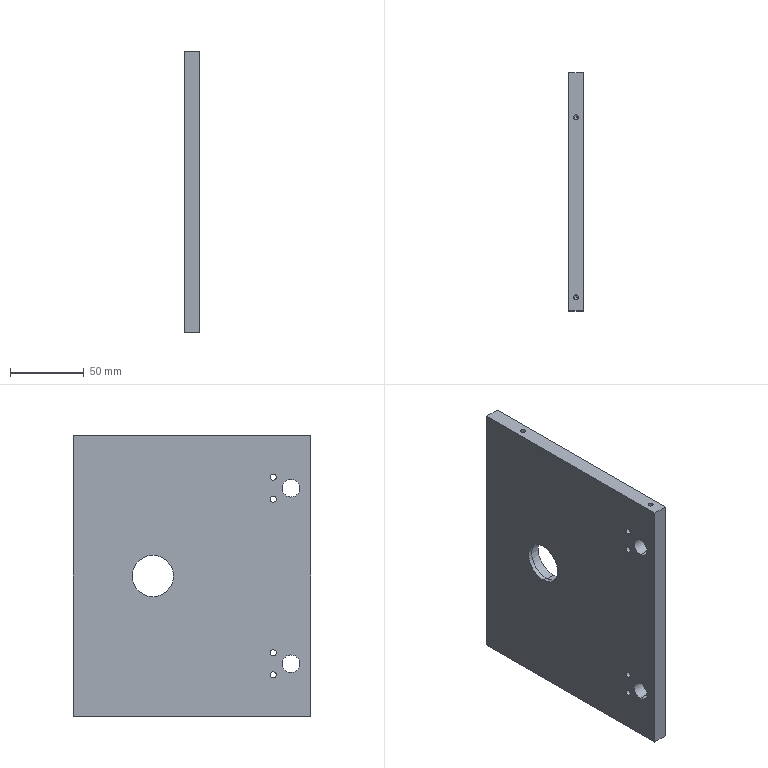Part | STEP file | 0245_216_Plate | 1 solid | 51 faces | box 10 x 161 x 190 mm | volume 295399 mm3 | cylinder 30 | cone 14 | plane 7 | commonest cylinder face diameters 4.2 x14 3.3 x8 12 x4 28 x2 30 x2